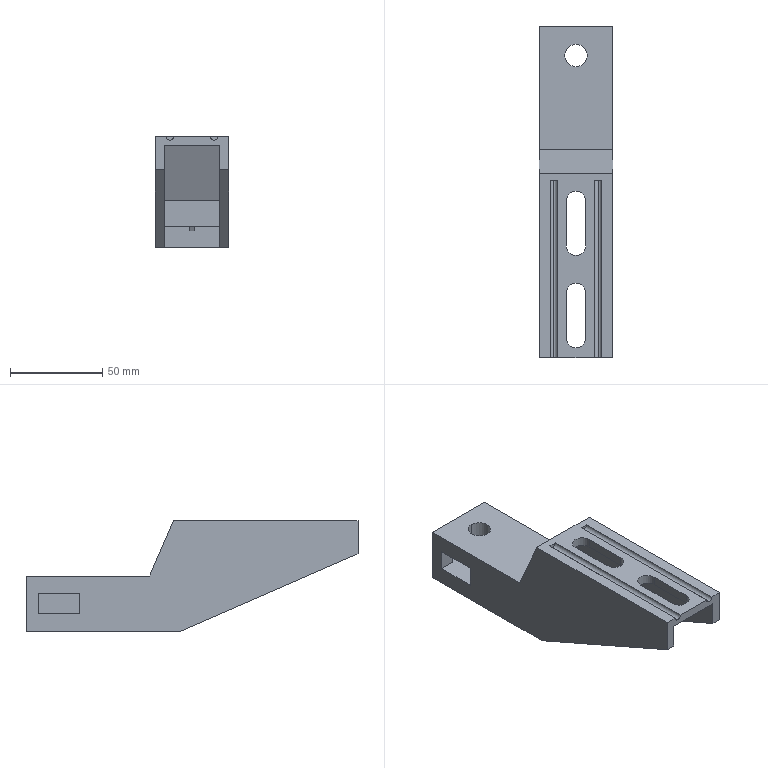Part | SolidWorks | features BaseBody 1 | 1 solid | 48 faces | box 40 x 180 x 60 mm | volume 106020 mm3 | plane 36 | cylinder 12 | commonest cylinder face diameters 4 x4 10.5 x4 12.2 x4
STEP:
#1=CARTESIAN_POINT('',(12.,96.,-2.));
#2=VERTEX_POINT('',#1);
#3=CARTESIAN_POINT('',(14.,96.,0.));
#4=VERTEX_POINT('',#3);
#5=CARTESIAN_POINT('',(12.,96.,0.));
#6=DIRECTION('',(0.,-1.,0.));
#7=DIRECTION('',(0.,0.,-1.));
#8=AXIS2_PLACEMENT_3D('',#5,#6,#7);
#9=CIRCLE('',#8,2.);
#10=EDGE_CURVE('',#2,#4,#9,.T.);
#11=ORIENTED_EDGE('',*,*,#10,.F.);
#12=CARTESIAN_POINT('',(12.,0.,-2.));
#13=VERTEX_POINT('',#12);
#14=CARTESIAN_POINT('',(12.,96.,-2.));
#15=DIRECTION('',(0.,-1.,0.));
#16=VECTOR('',#15,1000.);
#17=LINE('',#14,#16);
#18=EDGE_CURVE('',#2,#13,#17,.T.);
#19=ORIENTED_EDGE('',*,*,#18,.T.);
#20=CARTESIAN_POINT('',(14.,0.,0.));
#21=VERTEX_POINT('',#20);
#22=CARTESIAN_POINT('',(12.,0.,0.));
#23=DIRECTION('',(0.,-1.,0.));
#24=DIRECTION('',(0.,0.,-1.));
#25=AXIS2_PLACEMENT_3D('',#22,#23,#24);
#26=CIRCLE('',#25,2.);
#27=EDGE_CURVE('',#13,#21,#26,.T.);
#28=ORIENTED_EDGE('',*,*,#27,.T.);
#29=CARTESIAN_POINT('',(14.,0.,0.));
#30=DIRECTION('',(0.,1.,0.));
#31=VECTOR('',#30,1000.);
#32=LINE('',#29,#31);
#33=EDGE_CURVE('',#21,#4,#32,.T.);
#34=ORIENTED_EDGE('',*,*,#33,.T.);
#35=EDGE_LOOP('',(#11,#19,#28,#34));
#36=FACE_OUTER_BOUND('',#35,.T.);
#37=CARTESIAN_POINT('',(12.,96.,0.));
#38=DIRECTION('',(0.,-1.,0.));
#39=DIRECTION('',(0.,0.,-1.));
#40=AXIS2_PLACEMENT_3D('',#37,#38,#39);
#41=CYLINDRICAL_SURFACE('',#40,2.);
#42=ADVANCED_FACE('',(#36),#41,.F.);
#43=CARTESIAN_POINT('',(-12.,96.,-2.));
#44=VERTEX_POINT('',#43);
#45=CARTESIAN_POINT('',(-10.,96.,0.));
#46=VERTEX_POINT('',#45);
#47=CARTESIAN_POINT('',(-12.,96.,0.));
#48=DIRECTION('',(0.,-1.,0.));
#49=DIRECTION('',(0.,0.,-1.));
#50=AXIS2_PLACEMENT_3D('',#47,#48,#49);
#51=CIRCLE('',#50,2.);
#52=EDGE_CURVE('',#44,#46,#51,.T.);
#53=ORIENTED_EDGE('',*,*,#52,.F.);
#54=CARTESIAN_POINT('',(-12.,0.,-2.));
#55=VERTEX_POINT('',#54);
#56=CARTESIAN_POINT('',(-12.,96.,-2.));
#57=DIRECTION('',(0.,-1.,0.));
#58=VECTOR('',#57,1000.);
#59=LINE('',#56,#58);
#60=EDGE_CURVE('',#44,#55,#59,.T.);
#61=ORIENTED_EDGE('',*,*,#60,.T.);
#62=CARTESIAN_POINT('',(-10.,0.,0.));
#63=VERTEX_POINT('',#62);
#64=CARTESIAN_POINT('',(-12.,0.,0.));
#65=DIRECTION('',(0.,-1.,0.));
#66=DIRECTION('',(0.,0.,-1.));
#67=AXIS2_PLACEMENT_3D('',#64,#65,#66);
#68=CIRCLE('',#67,2.);
#69=EDGE_CURVE('',#55,#63,#68,.T.);
#70=ORIENTED_EDGE('',*,*,#69,.T.);
#71=CARTESIAN_POINT('',(-10.,0.,0.));
#72=DIRECTION('',(0.,1.,0.));
#73=VECTOR('',#72,1000.);
#74=LINE('',#71,#73);
#75=EDGE_CURVE('',#63,#46,#74,.T.);
#76=ORIENTED_EDGE('',*,*,#75,.T.);
#77=EDGE_LOOP('',(#53,#61,#70,#76));
#78=FACE_OUTER_BOUND('',#77,.T.);
#79=CARTESIAN_POINT('',(-12.,96.,0.));
#80=DIRECTION('',(0.,-1.,0.));
#81=DIRECTION('',(0.,0.,-1.));
#82=AXIS2_PLACEMENT_3D('',#79,#80,#81);
#83=CYLINDRICAL_SURFACE('',#82,2.);
#84=ADVANCED_FACE('',(#78),#83,.F.);
#85=CARTESIAN_POINT('',(0.,157.9,-50.6));
#86=VERTEX_POINT('',#85);
#87=CARTESIAN_POINT('',(0.,170.1,-50.6));
#88=VERTEX_POINT('',#87);
#89=CARTESIAN_POINT('',(0.,164.,-50.6));
#90=DIRECTION('',(0.,0.,-1.));
#91=DIRECTION('',(0.,1.,0.));
#92=AXIS2_PLACEMENT_3D('',#89,#90,#91);
#93=CIRCLE('',#92,6.1);
#94=EDGE_CURVE('',#86,#88,#93,.T.);
#95=ORIENTED_EDGE('',*,*,#94,.F.);
#96=CARTESIAN_POINT('',(0.,157.9,-60.));
#97=VERTEX_POINT('',#96);
#98=CARTESIAN_POINT('',(0.,157.9,0.));
#99=DIRECTION('',(0.,0.,-1.));
#100=VECTOR('',#99,1000.);
#101=LINE('',#98,#100);
#102=EDGE_CURVE('',#86,#97,#101,.T.);
#103=ORIENTED_EDGE('',*,*,#102,.T.);
#104=CARTESIAN_POINT('',(0.,170.1,-60.));
#105=VERTEX_POINT('',#104);
#106=CARTESIAN_POINT('',(0.,164.,-60.));
#107=DIRECTION('',(0.,0.,-1.));
#108=DIRECTION('',(0.,1.,0.));
#109=AXIS2_PLACEMENT_3D('',#106,#107,#108);
#110=CIRCLE('',#109,6.1);
#111=EDGE_CURVE('',#97,#105,#110,.T.);
#112=ORIENTED_EDGE('',*,*,#111,.T.);
#113=CARTESIAN_POINT('',(0.,170.1,0.));
#114=DIRECTION('',(0.,0.,-1.));
#115=VECTOR('',#114,1000.);
#116=LINE('',#113,#115);
#117=EDGE_CURVE('',#88,#105,#116,.T.);
#118=ORIENTED_EDGE('',*,*,#117,.F.);
#119=EDGE_LOOP('',(#95,#103,#112,#118));
#120=FACE_OUTER_BOUND('',#119,.T.);
#121=CARTESIAN_POINT('',(0.,164.,0.));
#122=DIRECTION('',(0.,0.,-1.));
#123=DIRECTION('',(0.,1.,0.));
#124=AXIS2_PLACEMENT_3D('',#121,#122,#123);
#125=CYLINDRICAL_SURFACE('',#124,6.1);
#126=ADVANCED_FACE('',(#120),#125,.F.);
#127=CARTESIAN_POINT('',(0.,170.1,-30.));
#128=VERTEX_POINT('',#127);
#129=CARTESIAN_POINT('',(0.,157.9,-30.));
#130=VERTEX_POINT('',#129);
#131=CARTESIAN_POINT('',(0.,164.,-30.));
#132=DIRECTION('',(0.,0.,1.));
#133=DIRECTION('',(0.,1.,0.));
#134=AXIS2_PLACEMENT_3D('',#131,#132,#133);
#135=CIRCLE('',#134,6.1);
#136=EDGE_CURVE('',#128,#130,#135,.T.);
#137=ORIENTED_EDGE('',*,*,#136,.T.);
#138=CARTESIAN_POINT('',(0.,157.9,-39.4));
#139=VERTEX_POINT('',#138);
#140=CARTESIAN_POINT('',(0.,157.9,0.));
#141=DIRECTION('',(0.,0.,-1.));
#142=VECTOR('',#141,1000.);
#143=LINE('',#140,#142);
#144=EDGE_CURVE('',#130,#139,#143,.T.);
#145=ORIENTED_EDGE('',*,*,#144,.T.);
#146=CARTESIAN_POINT('',(0.,170.1,-39.4));
#147=VERTEX_POINT('',#146);
#148=CARTESIAN_POINT('',(0.,164.,-39.4));
#149=DIRECTION('',(0.,0.,-1.));
#150=DIRECTION('',(0.,1.,0.));
#151=AXIS2_PLACEMENT_3D('',#148,#149,#150);
#152=CIRCLE('',#151,6.1);
#153=EDGE_CURVE('',#139,#147,#152,.T.);
#154=ORIENTED_EDGE('',*,*,#153,.T.);
#155=CARTESIAN_POINT('',(0.,170.1,0.));
#156=DIRECTION('',(0.,0.,-1.));
#157=VECTOR('',#156,1000.);
#158=LINE('',#155,#157);
#159=EDGE_CURVE('',#128,#147,#158,.T.);
#160=ORIENTED_EDGE('',*,*,#159,.F.);
#161=EDGE_LOOP('',(#137,#145,#154,#160));
#162=FACE_OUTER_BOUND('',#161,.T.);
#163=CARTESIAN_POINT('',(0.,164.,0.));
#164=DIRECTION('',(0.,0.,-1.));
#165=DIRECTION('',(0.,1.,0.));
#166=AXIS2_PLACEMENT_3D('',#163,#164,#165);
#167=CYLINDRICAL_SURFACE('',#166,6.1);
#168=ADVANCED_FACE('',(#162),#167,.F.);
#169=CARTESIAN_POINT('',(20.,96.,-60.));
#170=VERTEX_POINT('',#169);
#171=CARTESIAN_POINT('',(20.,0.,-18.));
#172=VERTEX_POINT('',#171);
#173=CARTESIAN_POINT('',(20.,96.,-60.));
#174=DIRECTION('',(0.,-0.9162,0.4008));
#175=VECTOR('',#174,1000.);
#176=LINE('',#173,#175);
#177=EDGE_CURVE('',#170,#172,#176,.T.);
#178=ORIENTED_EDGE('',*,*,#177,.F.);
#179=CARTESIAN_POINT('',(20.,180.,-60.));
#180=VERTEX_POINT('',#179);
#181=CARTESIAN_POINT('',(20.,0.,-60.));
#182=DIRECTION('',(0.,-1.,0.));
#183=VECTOR('',#182,1000.);
#184=LINE('',#181,#183);
#185=EDGE_CURVE('',#180,#170,#184,.T.);
#186=ORIENTED_EDGE('',*,*,#185,.F.);
#187=CARTESIAN_POINT('',(20.,180.,-30.));
#188=VERTEX_POINT('',#187);
#189=CARTESIAN_POINT('',(20.,180.,0.));
#190=DIRECTION('',(0.,0.,-1.));
#191=VECTOR('',#190,1000.);
#192=LINE('',#189,#191);
#193=EDGE_CURVE('',#188,#180,#192,.T.);
#194=ORIENTED_EDGE('',*,*,#193,.F.);
#195=CARTESIAN_POINT('',(20.,113.,-30.));
#196=VERTEX_POINT('',#195);
#197=CARTESIAN_POINT('',(20.,0.,-30.));
#198=DIRECTION('',(0.,1.,0.));
#199=VECTOR('',#198,1000.);
#200=LINE('',#197,#199);
#201=EDGE_CURVE('',#196,#188,#200,.T.);
#202=ORIENTED_EDGE('',*,*,#201,.F.);
#203=CARTESIAN_POINT('',(20.,100.,0.));
#204=VERTEX_POINT('',#203);
#205=CARTESIAN_POINT('',(20.,100.,0.));
#206=DIRECTION('',(0.,0.3976,-0.9176));
#207=VECTOR('',#206,1000.);
#208=LINE('',#205,#207);
#209=EDGE_CURVE('',#204,#196,#208,.T.);
#210=ORIENTED_EDGE('',*,*,#209,.F.);
#211=CARTESIAN_POINT('',(20.,0.,0.));
#212=VERTEX_POINT('',#211);
#213=CARTESIAN_POINT('',(20.,0.,0.));
#214=DIRECTION('',(0.,1.,0.));
#215=VECTOR('',#214,1000.);
#216=LINE('',#213,#215);
#217=EDGE_CURVE('',#212,#204,#216,.T.);
#218=ORIENTED_EDGE('',*,*,#217,.F.);
#219=CARTESIAN_POINT('',(20.,0.,0.));
#220=DIRECTION('',(0.,0.,1.));
#221=VECTOR('',#220,1000.);
#222=LINE('',#219,#221);
#223=EDGE_CURVE('',#172,#212,#222,.T.);
#224=ORIENTED_EDGE('',*,*,#223,.F.);
#225=EDGE_LOOP('',(#178,#186,#194,#202,#210,#218,#224));
#226=FACE_OUTER_BOUND('',#225,.T.);
#227=CARTESIAN_POINT('',(20.,0.,0.));
#228=DIRECTION('',(-1.,0.,0.));
#229=DIRECTION('',(0.,0.,1.));
#230=AXIS2_PLACEMENT_3D('',#227,#228,#229);
#231=PLANE('',#230);
#232=ADVANCED_FACE('',(#226),#231,.F.);
#233=CARTESIAN_POINT('',(10.,0.,0.));
#234=VERTEX_POINT('',#233);
#235=CARTESIAN_POINT('',(12.,0.,0.));
#236=DIRECTION('',(0.,-1.,0.));
#237=DIRECTION('',(0.,0.,-1.));
#238=AXIS2_PLACEMENT_3D('',#235,#236,#237);
#239=CIRCLE('',#238,2.);
#240=EDGE_CURVE('',#234,#13,#239,.T.);
#241=ORIENTED_EDGE('',*,*,#240,.F.);
#242=CARTESIAN_POINT('',(20.,0.,0.));
#243=DIRECTION('',(1.,0.,0.));
#244=VECTOR('',#243,1000.);
#245=LINE('',#242,#244);
#246=EDGE_CURVE('',#63,#234,#245,.T.);
#247=ORIENTED_EDGE('',*,*,#246,.F.);
#248=ORIENTED_EDGE('',*,*,#69,.F.);
#249=CARTESIAN_POINT('',(-14.,0.,0.));
#250=VERTEX_POINT('',#249);
#251=CARTESIAN_POINT('',(-12.,0.,0.));
#252=DIRECTION('',(0.,-1.,0.));
#253=DIRECTION('',(0.,0.,-1.));
#254=AXIS2_PLACEMENT_3D('',#251,#252,#253);
#255=CIRCLE('',#254,2.);
#256=EDGE_CURVE('',#250,#55,#255,.T.);
#257=ORIENTED_EDGE('',*,*,#256,.F.);
#258=CARTESIAN_POINT('',(-20.,0.,0.));
#259=VERTEX_POINT('',#258);
#260=CARTESIAN_POINT('',(20.,0.,0.));
#261=DIRECTION('',(1.,0.,0.));
#262=VECTOR('',#261,1000.);
#263=LINE('',#260,#262);
#264=EDGE_CURVE('',#259,#250,#263,.T.);
#265=ORIENTED_EDGE('',*,*,#264,.F.);
#266=CARTESIAN_POINT('',(-20.,0.,-18.));
#267=VERTEX_POINT('',#266);
#268=CARTESIAN_POINT('',(-20.,0.,-18.));
#269=DIRECTION('',(0.,0.,1.));
#270=VECTOR('',#269,1000.);
#271=LINE('',#268,#270);
#272=EDGE_CURVE('',#267,#259,#271,.T.);
#273=ORIENTED_EDGE('',*,*,#272,.F.);
#274=CARTESIAN_POINT('',(-15.,0.,-18.));
#275=VERTEX_POINT('',#274);
#276=CARTESIAN_POINT('',(20.,0.,-18.));
#277=DIRECTION('',(-1.,0.,0.));
#278=VECTOR('',#277,1000.);
#279=LINE('',#276,#278);
#280=EDGE_CURVE('',#275,#267,#279,.T.);
#281=ORIENTED_EDGE('',*,*,#280,.F.);
#282=CARTESIAN_POINT('',(-15.,0.,-5.));
#283=VERTEX_POINT('',#282);
#284=CARTESIAN_POINT('',(-15.,0.,-18.));
#285=DIRECTION('',(0.,0.,-1.));
#286=VECTOR('',#285,1000.);
#287=LINE('',#284,#286);
#288=EDGE_CURVE('',#283,#275,#287,.T.);
#289=ORIENTED_EDGE('',*,*,#288,.F.);
#290=CARTESIAN_POINT('',(15.,0.,-5.));
#291=VERTEX_POINT('',#290);
#292=CARTESIAN_POINT('',(20.,0.,-5.));
#293=DIRECTION('',(-1.,0.,0.));
#294=VECTOR('',#293,1000.);
#295=LINE('',#292,#294);
#296=EDGE_CURVE('',#291,#283,#295,.T.);
#297=ORIENTED_EDGE('',*,*,#296,.F.);
#298=CARTESIAN_POINT('',(15.,0.,-18.));
#299=VERTEX_POINT('',#298);
#300=CARTESIAN_POINT('',(15.,0.,-18.));
#301=DIRECTION('',(0.,0.,1.));
#302=VECTOR('',#301,1000.);
#303=LINE('',#300,#302);
#304=EDGE_CURVE('',#299,#291,#303,.T.);
#305=ORIENTED_EDGE('',*,*,#304,.F.);
#306=CARTESIAN_POINT('',(20.,0.,-18.));
#307=DIRECTION('',(-1.,0.,0.));
#308=VECTOR('',#307,1000.);
#309=LINE('',#306,#308);
#310=EDGE_CURVE('',#172,#299,#309,.T.);
#311=ORIENTED_EDGE('',*,*,#310,.F.);
#312=ORIENTED_EDGE('',*,*,#223,.T.);
#313=CARTESIAN_POINT('',(20.,0.,0.));
#314=DIRECTION('',(1.,0.,0.));
#315=VECTOR('',#314,1000.);
#316=LINE('',#313,#315);
#317=EDGE_CURVE('',#21,#212,#316,.T.);
#318=ORIENTED_EDGE('',*,*,#317,.F.);
#319=ORIENTED_EDGE('',*,*,#27,.F.);
#320=EDGE_LOOP('',(#241,#247,#248,#257,#265,#273,#281,#289,#297,#305,#311,#312,#318,#319));
#321=FACE_OUTER_BOUND('',#320,.T.);
#322=CARTESIAN_POINT('',(20.,0.,-18.));
#323=DIRECTION('',(0.,1.,0.));
#324=DIRECTION('',(0.,0.,1.));
#325=AXIS2_PLACEMENT_3D('',#322,#323,#324);
#326=PLANE('',#325);
#327=ADVANCED_FACE('',(#321),#326,.F.);
#328=CARTESIAN_POINT('',(15.,96.,-60.));
#329=VERTEX_POINT('',#328);
#330=CARTESIAN_POINT('',(15.,96.,-60.));
#331=DIRECTION('',(0.,-0.9162,0.4008));
#332=VECTOR('',#331,1000.);
#333=LINE('',#330,#332);
#334=EDGE_CURVE('',#329,#299,#333,.T.);
#335=ORIENTED_EDGE('',*,*,#334,.F.);
#336=CARTESIAN_POINT('',(20.,96.,-60.));
#337=DIRECTION('',(-1.,0.,0.));
#338=VECTOR('',#337,1000.);
#339=LINE('',#336,#338);
#340=EDGE_CURVE('',#170,#329,#339,.T.);
#341=ORIENTED_EDGE('',*,*,#340,.F.);
#342=ORIENTED_EDGE('',*,*,#177,.T.);
#343=ORIENTED_EDGE('',*,*,#310,.T.);
#344=EDGE_LOOP('',(#335,#341,#342,#343));
#345=FACE_OUTER_BOUND('',#344,.T.);
#346=CARTESIAN_POINT('',(20.,96.,-60.));
#347=DIRECTION('',(0.,0.4008,0.9162));
#348=DIRECTION('',(0.,-0.9162,0.4008));
#349=AXIS2_PLACEMENT_3D('',#346,#347,#348);
#350=PLANE('',#349);
#351=ADVANCED_FACE('',(#345),#350,.F.);
#352=CARTESIAN_POINT('',(0.,164.,-60.));
#353=DIRECTION('',(0.,0.,-1.));
#354=DIRECTION('',(0.,1.,0.));
#355=AXIS2_PLACEMENT_3D('',#352,#353,#354);
#356=CIRCLE('',#355,6.1);
#357=EDGE_CURVE('',#105,#97,#356,.T.);
#358=ORIENTED_EDGE('',*,*,#357,.F.);
#359=ORIENTED_EDGE('',*,*,#111,.F.);
#360=EDGE_LOOP('',(#358,#359));
#361=FACE_BOUND('',#360,.T.);
#362=CARTESIAN_POINT('',(-20.,96.,-60.));
#363=VERTEX_POINT('',#362);
#364=CARTESIAN_POINT('',(-15.,96.,-60.));
#365=VERTEX_POINT('',#364);
#366=CARTESIAN_POINT('',(20.,96.,-60.));
#367=DIRECTION('',(1.,0.,0.));
#368=VECTOR('',#367,1000.);
#369=LINE('',#366,#368);
#370=EDGE_CURVE('',#363,#365,#369,.T.);
#371=ORIENTED_EDGE('',*,*,#370,.F.);
#372=CARTESIAN_POINT('',(-20.,180.,-60.));
#373=VERTEX_POINT('',#372);
#374=CARTESIAN_POINT('',(-20.,180.,-60.));
#375=DIRECTION('',(0.,-1.,0.));
#376=VECTOR('',#375,1000.);
#377=LINE('',#374,#376);
#378=EDGE_CURVE('',#373,#363,#377,.T.);
#379=ORIENTED_EDGE('',*,*,#378,.F.);
#380=CARTESIAN_POINT('',(20.,180.,-60.));
#381=DIRECTION('',(-1.,0.,0.));
#382=VECTOR('',#381,1000.);
#383=LINE('',#380,#382);
#384=EDGE_CURVE('',#180,#373,#383,.T.);
#385=ORIENTED_EDGE('',*,*,#384,.F.);
#386=ORIENTED_EDGE('',*,*,#185,.T.);
#387=ORIENTED_EDGE('',*,*,#340,.T.);
#388=CARTESIAN_POINT('',(15.,147.,-60.));
#389=VERTEX_POINT('',#388);
#390=CARTESIAN_POINT('',(15.,180.,-60.));
#391=DIRECTION('',(0.,-1.,0.));
#392=VECTOR('',#391,1000.);
#393=LINE('',#390,#392);
#394=EDGE_CURVE('',#389,#329,#393,.T.);
#395=ORIENTED_EDGE('',*,*,#394,.F.);
#396=CARTESIAN_POINT('',(-15.,147.,-60.));
#397=VERTEX_POINT('',#396);
#398=CARTESIAN_POINT('',(20.,147.,-60.));
#399=DIRECTION('',(1.,0.,0.));
#400=VECTOR('',#399,1000.);
#401=LINE('',#398,#400);
#402=EDGE_CURVE('',#397,#389,#401,.T.);
#403=ORIENTED_EDGE('',*,*,#402,.F.);
#404=CARTESIAN_POINT('',(-15.,180.,-60.));
#405=DIRECTION('',(0.,1.,0.));
#406=VECTOR('',#405,1000.);
#407=LINE('',#404,#406);
#408=EDGE_CURVE('',#365,#397,#407,.T.);
#409=ORIENTED_EDGE('',*,*,#408,.F.);
#410=EDGE_LOOP('',(#371,#379,#385,#386,#387,#395,#403,#409));
#411=FACE_OUTER_BOUND('',#410,.T.);
#412=CARTESIAN_POINT('',(20.,180.,-60.));
#413=DIRECTION('',(0.,0.,1.));
#414=DIRECTION('',(0.,-1.,0.));
#415=AXIS2_PLACEMENT_3D('',#412,#413,#414);
#416=PLANE('',#415);
#417=ADVANCED_FACE('',(#361,#411),#416,.F.);
#418=CARTESIAN_POINT('',(-11.5,180.,-50.6));
#419=VERTEX_POINT('',#418);
#420=CARTESIAN_POINT('',(-11.5,180.,-39.4));
#421=VERTEX_POINT('',#420);
#422=CARTESIAN_POINT('',(-11.5,180.,-30.));
#423=DIRECTION('',(0.,0.,1.));
#424=VECTOR('',#423,1000.);
#425=LINE('',#422,#424);
#426=EDGE_CURVE('',#419,#421,#425,.T.);
#427=ORIENTED_EDGE('',*,*,#426,.F.);
#428=CARTESIAN_POINT('',(11.5,180.,-50.6));
#429=VERTEX_POINT('',#428);
#430=CARTESIAN_POINT('',(20.,180.,-50.6));
#431=DIRECTION('',(-1.,0.,0.));
#432=VECTOR('',#431,1000.);
#433=LINE('',#430,#432);
#434=EDGE_CURVE('',#429,#419,#433,.T.);
#435=ORIENTED_EDGE('',*,*,#434,.F.);
#436=CARTESIAN_POINT('',(11.5,180.,-39.4));
#437=VERTEX_POINT('',#436);
#438=CARTESIAN_POINT('',(11.5,180.,-30.));
#439=DIRECTION('',(0.,0.,-1.));
#440=VECTOR('',#439,1000.);
#441=LINE('',#438,#440);
#442=EDGE_CURVE('',#437,#429,#441,.T.);
#443=ORIENTED_EDGE('',*,*,#442,.F.);
#444=CARTESIAN_POINT('',(20.,180.,-39.4));
#445=DIRECTION('',(1.,0.,0.));
#446=VECTOR('',#445,1000.);
#447=LINE('',#444,#446);
#448=EDGE_CURVE('',#421,#437,#447,.T.);
#449=ORIENTED_EDGE('',*,*,#448,.F.);
#450=EDGE_LOOP('',(#427,#435,#443,#449));
#451=FACE_BOUND('',#450,.T.);
#452=CARTESIAN_POINT('',(-20.,180.,-30.));
#453=VERTEX_POINT('',#452);
#454=CARTESIAN_POINT('',(20.,180.,-30.));
#455=DIRECTION('',(-1.,0.,0.));
#456=VECTOR('',#455,1000.);
#457=LINE('',#454,#456);
#458=EDGE_CURVE('',#188,#453,#457,.T.);
#459=ORIENTED_EDGE('',*,*,#458,.F.);
#460=ORIENTED_EDGE('',*,*,#193,.T.);
#461=ORIENTED_EDGE('',*,*,#384,.T.);
#462=CARTESIAN_POINT('',(-20.,180.,-30.));
#463=DIRECTION('',(0.,0.,-1.));
#464=VECTOR('',#463,1000.);
#465=LINE('',#462,#464);
#466=EDGE_CURVE('',#453,#373,#465,.T.);
#467=ORIENTED_EDGE('',*,*,#466,.F.);
#468=EDGE_LOOP('',(#459,#460,#461,#467));
#469=FACE_OUTER_BOUND('',#468,.T.);
#470=CARTESIAN_POINT('',(20.,180.,-30.));
#471=DIRECTION('',(0.,-1.,0.));
#472=DIRECTION('',(0.,0.,-1.));
#473=AXIS2_PLACEMENT_3D('',#470,#471,#472);
#474=PLANE('',#473);
#475=ADVANCED_FACE('',(#451,#469),#474,.F.);
#476=ORIENTED_EDGE('',*,*,#136,.F.);
#477=CARTESIAN_POINT('',(0.,164.,-30.));
#478=DIRECTION('',(0.,0.,1.));
#479=DIRECTION('',(0.,1.,0.));
#480=AXIS2_PLACEMENT_3D('',#477,#478,#479);
#481=CIRCLE('',#480,6.1);
#482=EDGE_CURVE('',#130,#128,#481,.T.);
#483=ORIENTED_EDGE('',*,*,#482,.F.);
#484=EDGE_LOOP('',(#476,#483));
#485=FACE_BOUND('',#484,.T.);
#486=CARTESIAN_POINT('',(-20.,113.,-30.));
#487=VERTEX_POINT('',#486);
#488=CARTESIAN_POINT('',(20.,113.,-30.));
#489=DIRECTION('',(-1.,0.,0.));
#490=VECTOR('',#489,1000.);
#491=LINE('',#488,#490);
#492=EDGE_CURVE('',#196,#487,#491,.T.);
#493=ORIENTED_EDGE('',*,*,#492,.F.);
#494=ORIENTED_EDGE('',*,*,#201,.T.);
#495=ORIENTED_EDGE('',*,*,#458,.T.);
#496=CARTESIAN_POINT('',(-20.,113.,-30.));
#497=DIRECTION('',(0.,1.,0.));
#498=VECTOR('',#497,1000.);
#499=LINE('',#496,#498);
#500=EDGE_CURVE('',#487,#453,#499,.T.);
#501=ORIENTED_EDGE('',*,*,#500,.F.);
#502=EDGE_LOOP('',(#493,#494,#495,#501));
#503=FACE_OUTER_BOUND('',#502,.T.);
#504=CARTESIAN_POINT('',(20.,113.,-30.));
#505=DIRECTION('',(0.,0.,-1.));
#506=DIRECTION('',(-1.,0.,0.));
#507=AXIS2_PLACEMENT_3D('',#504,#505,#506);
#508=PLANE('',#507);
#509=ADVANCED_FACE('',(#485,#503),#508,.F.);
#510=CARTESIAN_POINT('',(-20.,100.,0.));
#511=VERTEX_POINT('',#510);
#512=CARTESIAN_POINT('',(20.,100.,0.));
#513=DIRECTION('',(-1.,0.,0.));
#514=VECTOR('',#513,1000.);
#515=LINE('',#512,#514);
#516=EDGE_CURVE('',#204,#511,#515,.T.);
#517=ORIENTED_EDGE('',*,*,#516,.F.);
#518=ORIENTED_EDGE('',*,*,#209,.T.);
#519=ORIENTED_EDGE('',*,*,#492,.T.);
#520=CARTESIAN_POINT('',(-20.,100.,0.));
#521=DIRECTION('',(0.,0.3976,-0.9176));
#522=VECTOR('',#521,1000.);
#523=LINE('',#520,#522);
#524=EDGE_CURVE('',#511,#487,#523,.T.);
#525=ORIENTED_EDGE('',*,*,#524,.F.);
#526=EDGE_LOOP('',(#517,#518,#519,#525));
#527=FACE_OUTER_BOUND('',#526,.T.);
#528=CARTESIAN_POINT('',(20.,100.,0.));
#529=DIRECTION('',(0.,-0.9176,-0.3976));
#530=DIRECTION('',(0.,0.3976,-0.9176));
#531=AXIS2_PLACEMENT_3D('',#528,#529,#530);
#532=PLANE('',#531);
#533=ADVANCED_FACE('',(#527),#532,.F.);
#534=CARTESIAN_POINT('',(-5.25,10.75,0.));
#535=VERTEX_POINT('',#534);
#536=CARTESIAN_POINT('',(5.25,10.75,0.));
#537=VERTEX_POINT('',#536);
#538=CARTESIAN_POINT('',(0.,10.75,0.));
#539=DIRECTION('',(0.,0.,1.));
#540=DIRECTION('',(1.,0.,0.));
#541=AXIS2_PLACEMENT_3D('',#538,#539,#540);
#542=CIRCLE('',#541,5.25);
#543=EDGE_CURVE('',#535,#537,#542,.T.);
#544=ORIENTED_EDGE('',*,*,#543,.F.);
#545=CARTESIAN_POINT('',(-5.25,35.25,0.));
#546=VERTEX_POINT('',#545);
#547=CARTESIAN_POINT('',(-5.25,0.,0.));
#548=DIRECTION('',(0.,-1.,0.));
#549=VECTOR('',#548,1000.);
#550=LINE('',#547,#549);
#551=EDGE_CURVE('',#546,#535,#550,.T.);
#552=ORIENTED_EDGE('',*,*,#551,.F.);
#553=CARTESIAN_POINT('',(5.25,35.25,0.));
#554=VERTEX_POINT('',#553);
#555=CARTESIAN_POINT('',(0.,35.25,0.));
#556=DIRECTION('',(0.,0.,1.));
#557=DIRECTION('',(1.,0.,0.));
#558=AXIS2_PLACEMENT_3D('',#555,#556,#557);
#559=CIRCLE('',#558,5.25);
#560=EDGE_CURVE('',#554,#546,#559,.T.);
#561=ORIENTED_EDGE('',*,*,#560,.F.);
#562=CARTESIAN_POINT('',(5.25,0.,0.));
#563=DIRECTION('',(0.,1.,0.));
#564=VECTOR('',#563,1000.);
#565=LINE('',#562,#564);
#566=EDGE_CURVE('',#537,#554,#565,.T.);
#567=ORIENTED_EDGE('',*,*,#566,.F.);
#568=EDGE_LOOP('',(#544,#552,#561,#567));
#569=FACE_BOUND('',#568,.T.);
#570=CARTESIAN_POINT('',(-5.25,60.75,0.));
#571=VERTEX_POINT('',#570);
#572=CARTESIAN_POINT('',(5.25,60.75,0.));
#573=VERTEX_POINT('',#572);
#574=CARTESIAN_POINT('',(0.,60.75,0.));
#575=DIRECTION('',(0.,0.,1.));
#576=DIRECTION('',(1.,0.,0.));
#577=AXIS2_PLACEMENT_3D('',#574,#575,#576);
#578=CIRCLE('',#577,5.25);
#579=EDGE_CURVE('',#571,#573,#578,.T.);
#580=ORIENTED_EDGE('',*,*,#579,.F.);
#581=CARTESIAN_POINT('',(-5.25,85.25,0.));
#582=VERTEX_POINT('',#581);
#583=CARTESIAN_POINT('',(-5.25,0.,0.));
#584=DIRECTION('',(0.,-1.,0.));
#585=VECTOR('',#584,1000.);
#586=LINE('',#583,#585);
#587=EDGE_CURVE('',#582,#571,#586,.T.);
#588=ORIENTED_EDGE('',*,*,#587,.F.);
#589=CARTESIAN_POINT('',(5.25,85.25,0.));
#590=VERTEX_POINT('',#589);
#591=CARTESIAN_POINT('',(0.,85.25,0.));
#592=DIRECTION('',(0.,0.,1.));
#593=DIRECTION('',(1.,0.,0.));
#594=AXIS2_PLACEMENT_3D('',#591,#592,#593);
#595=CIRCLE('',#594,5.25);
#596=EDGE_CURVE('',#590,#582,#595,.T.);
#597=ORIENTED_EDGE('',*,*,#596,.F.);
#598=CARTESIAN_POINT('',(5.25,0.,0.));
#599=DIRECTION('',(0.,1.,0.));
#600=VECTOR('',#599,1000.);
#601=LINE('',#598,#600);
#602=EDGE_CURVE('',#573,#590,#601,.T.);
#603=ORIENTED_EDGE('',*,*,#602,.F.);
#604=EDGE_LOOP('',(#580,#588,#597,#603));
#605=FACE_BOUND('',#604,.T.);
#606=ORIENTED_EDGE('',*,*,#33,.F.);
#607=ORIENTED_EDGE('',*,*,#317,.T.);
#608=ORIENTED_EDGE('',*,*,#217,.T.);
#609=ORIENTED_EDGE('',*,*,#516,.T.);
#610=CARTESIAN_POINT('',(-20.,0.,0.));
#611=DIRECTION('',(0.,1.,0.));
#612=VECTOR('',#611,1000.);
#613=LINE('',#610,#612);
#614=EDGE_CURVE('',#259,#511,#613,.T.);
#615=ORIENTED_EDGE('',*,*,#614,.F.);
#616=ORIENTED_EDGE('',*,*,#264,.T.);
#617=CARTESIAN_POINT('',(-14.,96.,0.));
#618=VERTEX_POINT('',#617);
#619=CARTESIAN_POINT('',(-14.,0.,0.));
#620=DIRECTION('',(0.,-1.,0.));
#621=VECTOR('',#620,1000.);
#622=LINE('',#619,#621);
#623=EDGE_CURVE('',#618,#250,#622,.T.);
#624=ORIENTED_EDGE('',*,*,#623,.F.);
#625=CARTESIAN_POINT('',(20.,96.,0.));
#626=DIRECTION('',(-1.,0.,0.));
#627=VECTOR('',#626,1000.);
#628=LINE('',#625,#627);
#629=EDGE_CURVE('',#46,#618,#628,.T.);
#630=ORIENTED_EDGE('',*,*,#629,.F.);
#631=ORIENTED_EDGE('',*,*,#75,.F.);
#632=ORIENTED_EDGE('',*,*,#246,.T.);
#633=CARTESIAN_POINT('',(10.,96.,0.));
#634=VERTEX_POINT('',#633);
#635=CARTESIAN_POINT('',(10.,0.,0.));
#636=DIRECTION('',(0.,-1.,0.));
#637=VECTOR('',#636,1000.);
#638=LINE('',#635,#637);
#639=EDGE_CURVE('',#634,#234,#638,.T.);
#640=ORIENTED_EDGE('',*,*,#639,.F.);
#641=CARTESIAN_POINT('',(20.,96.,0.));
#642=DIRECTION('',(-1.,0.,0.));
#643=VECTOR('',#642,1000.);
#644=LINE('',#641,#643);
#645=EDGE_CURVE('',#4,#634,#644,.T.);
#646=ORIENTED_EDGE('',*,*,#645,.F.);
#647=EDGE_LOOP('',(#606,#607,#608,#609,#615,#616,#624,#630,#631,#632,#640,#646));
#648=FACE_OUTER_BOUND('',#647,.T.);
#649=CARTESIAN_POINT('',(20.,0.,0.));
#650=DIRECTION('',(0.,0.,-1.));
#651=DIRECTION('',(-1.,0.,0.));
#652=AXIS2_PLACEMENT_3D('',#649,#650,#651);
#653=PLANE('',#652);
#654=ADVANCED_FACE('',(#569,#605,#648),#653,.F.);
#655=ORIENTED_EDGE('',*,*,#18,.F.);
#656=CARTESIAN_POINT('',(12.,96.,0.));
#657=DIRECTION('',(0.,-1.,0.));
#658=DIRECTION('',(0.,0.,-1.));
#659=AXIS2_PLACEMENT_3D('',#656,#657,#658);
#660=CIRCLE('',#659,2.);
#661=EDGE_CURVE('',#634,#2,#660,.T.);
#662=ORIENTED_EDGE('',*,*,#661,.F.);
#663=ORIENTED_EDGE('',*,*,#639,.T.);
#664=ORIENTED_EDGE('',*,*,#240,.T.);
#665=EDGE_LOOP('',(#655,#662,#663,#664));
#666=FACE_OUTER_BOUND('',#665,.T.);
#667=CARTESIAN_POINT('',(12.,96.,0.));
#668=DIRECTION('',(0.,-1.,0.));
#669=DIRECTION('',(0.,0.,-1.));
#670=AXIS2_PLACEMENT_3D('',#667,#668,#669);
#671=CYLINDRICAL_SURFACE('',#670,2.);
#672=ADVANCED_FACE('',(#666),#671,.F.);
#673=ORIENTED_EDGE('',*,*,#60,.F.);
#674=CARTESIAN_POINT('',(-12.,96.,0.));
#675=DIRECTION('',(0.,-1.,0.));
#676=DIRECTION('',(0.,0.,-1.));
#677=AXIS2_PLACEMENT_3D('',#674,#675,#676);
#678=CIRCLE('',#677,2.);
#679=EDGE_CURVE('',#618,#44,#678,.T.);
#680=ORIENTED_EDGE('',*,*,#679,.F.);
#681=ORIENTED_EDGE('',*,*,#623,.T.);
#682=ORIENTED_EDGE('',*,*,#256,.T.);
#683=EDGE_LOOP('',(#673,#680,#681,#682));
#684=FACE_OUTER_BOUND('',#683,.T.);
#685=CARTESIAN_POINT('',(-12.,96.,0.));
#686=DIRECTION('',(0.,-1.,0.));
#687=DIRECTION('',(0.,0.,-1.));
#688=AXIS2_PLACEMENT_3D('',#685,#686,#687);
#689=CYLINDRICAL_SURFACE('',#688,2.);
#690=ADVANCED_FACE('',(#684),#689,.F.);
#691=CARTESIAN_POINT('',(-20.,173.,-39.4));
#692=VERTEX_POINT('',#691);
#693=CARTESIAN_POINT('',(-20.,151.,-39.4));
#694=VERTEX_POINT('',#693);
#695=CARTESIAN_POINT('',(-20.,0.,-39.4));
#696=DIRECTION('',(0.,-1.,0.));
#697=VECTOR('',#696,1000.);
#698=LINE('',#695,#697);
#699=EDGE_CURVE('',#692,#694,#698,.T.);
#700=ORIENTED_EDGE('',*,*,#699,.T.);
#701=CARTESIAN_POINT('',(-20.,151.,-50.6));
#702=VERTEX_POINT('',#701);
#703=CARTESIAN_POINT('',(-20.,151.,0.));
#704=DIRECTION('',(0.,0.,-1.));
#705=VECTOR('',#704,1000.);
#706=LINE('',#703,#705);
#707=EDGE_CURVE('',#694,#702,#706,.T.);
#708=ORIENTED_EDGE('',*,*,#707,.T.);
#709=CARTESIAN_POINT('',(-20.,173.,-50.6));
#710=VERTEX_POINT('',#709);
#711=CARTESIAN_POINT('',(-20.,0.,-50.6));
#712=DIRECTION('',(0.,1.,0.));
#713=VECTOR('',#712,1000.);
#714=LINE('',#711,#713);
#715=EDGE_CURVE('',#702,#710,#714,.T.);
#716=ORIENTED_EDGE('',*,*,#715,.T.);
#717=CARTESIAN_POINT('',(-20.,173.,0.));
#718=DIRECTION('',(0.,0.,1.));
#719=VECTOR('',#718,1000.);
#720=LINE('',#717,#719);
#721=EDGE_CURVE('',#710,#692,#720,.T.);
#722=ORIENTED_EDGE('',*,*,#721,.T.);
#723=EDGE_LOOP('',(#700,#708,#716,#722));
#724=FACE_BOUND('',#723,.T.);
#725=ORIENTED_EDGE('',*,*,#378,.T.);
#726=CARTESIAN_POINT('',(-20.,96.,-60.));
#727=DIRECTION('',(0.,-0.9162,0.4008));
#728=VECTOR('',#727,1000.);
#729=LINE('',#726,#728);
#730=EDGE_CURVE('',#363,#267,#729,.T.);
#731=ORIENTED_EDGE('',*,*,#730,.T.);
#732=ORIENTED_EDGE('',*,*,#272,.T.);
#733=ORIENTED_EDGE('',*,*,#614,.T.);
#734=ORIENTED_EDGE('',*,*,#524,.T.);
#735=ORIENTED_EDGE('',*,*,#500,.T.);
#736=ORIENTED_EDGE('',*,*,#466,.T.);
#737=EDGE_LOOP('',(#725,#731,#732,#733,#734,#735,#736));
#738=FACE_OUTER_BOUND('',#737,.T.);
#739=CARTESIAN_POINT('',(-20.,0.,0.));
#740=DIRECTION('',(-1.,0.,0.));
#741=DIRECTION('',(0.,0.,1.));
#742=AXIS2_PLACEMENT_3D('',#739,#740,#741);
#743=PLANE('',#742);
#744=ADVANCED_FACE('',(#724,#738),#743,.T.);
#745=ORIENTED_EDGE('',*,*,#280,.T.);
#746=ORIENTED_EDGE('',*,*,#730,.F.);
#747=ORIENTED_EDGE('',*,*,#370,.T.);
#748=CARTESIAN_POINT('',(-15.,96.,-60.));
#749=DIRECTION('',(0.,0.9162,-0.4008));
#750=VECTOR('',#749,1000.);
#751=LINE('',#748,#750);
#752=EDGE_CURVE('',#275,#365,#751,.T.);
#753=ORIENTED_EDGE('',*,*,#752,.F.);
#754=EDGE_LOOP('',(#745,#746,#747,#753));
#755=FACE_OUTER_BOUND('',#754,.T.);
#756=CARTESIAN_POINT('',(20.,96.,-60.));
#757=DIRECTION('',(0.,0.4008,0.9162));
#758=DIRECTION('',(0.,-0.9162,0.4008));
#759=AXIS2_PLACEMENT_3D('',#756,#757,#758);
#760=PLANE('',#759);
#761=ADVANCED_FACE('',(#755),#760,.F.);
#762=CARTESIAN_POINT('',(-15.,109.4,-48.633));
#763=VERTEX_POINT('',#762);
#764=CARTESIAN_POINT('',(-15.,111.6,-48.633));
#765=VERTEX_POINT('',#764);
#766=CARTESIAN_POINT('',(-15.,0.,-48.633));
#767=DIRECTION('',(0.,1.,0.));
#768=VECTOR('',#767,1000.);
#769=LINE('',#766,#768);
#770=EDGE_CURVE('',#763,#765,#769,.T.);
#771=ORIENTED_EDGE('',*,*,#770,.F.);
#772=CARTESIAN_POINT('',(-15.,109.4,-34.633));
#773=VERTEX_POINT('',#772);
#774=CARTESIAN_POINT('',(-15.,109.4,0.));
#775=DIRECTION('',(0.,0.,-1.));
#776=VECTOR('',#775,1000.);
#777=LINE('',#774,#776);
#778=EDGE_CURVE('',#773,#763,#777,.T.);
#779=ORIENTED_EDGE('',*,*,#778,.F.);
#780=CARTESIAN_POINT('',(-15.,109.558,-34.633));
#781=VERTEX_POINT('',#780);
#782=CARTESIAN_POINT('',(-15.,111.6,-34.633));
#783=DIRECTION('',(0.,-1.,0.));
#784=VECTOR('',#783,1000.);
#785=LINE('',#782,#784);
#786=EDGE_CURVE('',#781,#773,#785,.T.);
#787=ORIENTED_EDGE('',*,*,#786,.F.);
#788=CARTESIAN_POINT('',(-15.,96.717,-5.));
#789=VERTEX_POINT('',#788);
#790=CARTESIAN_POINT('',(-15.,96.717,-5.));
#791=DIRECTION('',(0.,0.3976,-0.9176));
#792=VECTOR('',#791,1000.);
#793=LINE('',#790,#792);
#794=EDGE_CURVE('',#789,#781,#793,.T.);
#795=ORIENTED_EDGE('',*,*,#794,.F.);
#796=CARTESIAN_POINT('',(-15.,0.,-5.));
#797=DIRECTION('',(0.,1.,0.));
#798=VECTOR('',#797,1000.);
#799=LINE('',#796,#798);
#800=EDGE_CURVE('',#283,#789,#799,.T.);
#801=ORIENTED_EDGE('',*,*,#800,.F.);
#802=ORIENTED_EDGE('',*,*,#288,.T.);
#803=ORIENTED_EDGE('',*,*,#752,.T.);
#804=ORIENTED_EDGE('',*,*,#408,.T.);
#805=CARTESIAN_POINT('',(-15.,147.,-35.));
#806=VERTEX_POINT('',#805);
#807=CARTESIAN_POINT('',(-15.,147.,0.));
#808=DIRECTION('',(0.,0.,-1.));
#809=VECTOR('',#808,1000.);
#810=LINE('',#807,#809);
#811=EDGE_CURVE('',#806,#397,#810,.T.);
#812=ORIENTED_EDGE('',*,*,#811,.F.);
#813=CARTESIAN_POINT('',(-15.,111.6,-35.));
#814=VERTEX_POINT('',#813);
#815=CARTESIAN_POINT('',(-15.,0.,-35.));
#816=DIRECTION('',(0.,1.,0.));
#817=VECTOR('',#816,1000.);
#818=LINE('',#815,#817);
#819=EDGE_CURVE('',#814,#806,#818,.T.);
#820=ORIENTED_EDGE('',*,*,#819,.F.);
#821=CARTESIAN_POINT('',(-15.,111.6,0.));
#822=DIRECTION('',(0.,0.,1.));
#823=VECTOR('',#822,1000.);
#824=LINE('',#821,#823);
#825=EDGE_CURVE('',#765,#814,#824,.T.);
#826=ORIENTED_EDGE('',*,*,#825,.F.);
#827=EDGE_LOOP('',(#771,#779,#787,#795,#801,#802,#803,#804,#812,#820,#826));
#828=FACE_OUTER_BOUND('',#827,.T.);
#829=CARTESIAN_POINT('',(-15.,0.,0.));
#830=DIRECTION('',(-1.,0.,0.));
#831=DIRECTION('',(0.,0.,1.));
#832=AXIS2_PLACEMENT_3D('',#829,#830,#831);
#833=PLANE('',#832);
#834=ADVANCED_FACE('',(#828),#833,.F.);
#835=CARTESIAN_POINT('',(5.25,35.25,-5.));
#836=VERTEX_POINT('',#835);
#837=CARTESIAN_POINT('',(-5.25,35.25,-5.));
#838=VERTEX_POINT('',#837);
#839=CARTESIAN_POINT('',(0.,35.25,-5.));
#840=DIRECTION('',(0.,0.,1.));
#841=DIRECTION('',(1.,0.,0.));
#842=AXIS2_PLACEMENT_3D('',#839,#840,#841);
#843=CIRCLE('',#842,5.25);
#844=EDGE_CURVE('',#836,#838,#843,.T.);
#845=ORIENTED_EDGE('',*,*,#844,.T.);
#846=CARTESIAN_POINT('',(-5.25,10.75,-5.));
#847=VERTEX_POINT('',#846);
#848=CARTESIAN_POINT('',(-5.25,0.,-5.));
#849=DIRECTION('',(0.,-1.,0.));
#850=VECTOR('',#849,1000.);
#851=LINE('',#848,#850);
#852=EDGE_CURVE('',#838,#847,#851,.T.);
#853=ORIENTED_EDGE('',*,*,#852,.T.);
#854=CARTESIAN_POINT('',(5.25,10.75,-5.));
#855=VERTEX_POINT('',#854);
#856=CARTESIAN_POINT('',(0.,10.75,-5.));
#857=DIRECTION('',(0.,0.,1.));
#858=DIRECTION('',(1.,0.,0.));
#859=AXIS2_PLACEMENT_3D('',#856,#857,#858);
#860=CIRCLE('',#859,5.25);
#861=EDGE_CURVE('',#847,#855,#860,.T.);
#862=ORIENTED_EDGE('',*,*,#861,.T.);
#863=CARTESIAN_POINT('',(5.25,0.,-5.));
#864=DIRECTION('',(0.,1.,0.));
#865=VECTOR('',#864,1000.);
#866=LINE('',#863,#865);
#867=EDGE_CURVE('',#855,#836,#866,.T.);
#868=ORIENTED_EDGE('',*,*,#867,.T.);
#869=EDGE_LOOP('',(#845,#853,#862,#868));
#870=FACE_BOUND('',#869,.T.);
#871=CARTESIAN_POINT('',(5.25,85.25,-5.));
#872=VERTEX_POINT('',#871);
#873=CARTESIAN_POINT('',(-5.25,85.25,-5.));
#874=VERTEX_POINT('',#873);
#875=CARTESIAN_POINT('',(0.,85.25,-5.));
#876=DIRECTION('',(0.,0.,1.));
#877=DIRECTION('',(1.,0.,0.));
#878=AXIS2_PLACEMENT_3D('',#875,#876,#877);
#879=CIRCLE('',#878,5.25);
#880=EDGE_CURVE('',#872,#874,#879,.T.);
#881=ORIENTED_EDGE('',*,*,#880,.T.);
#882=CARTESIAN_POINT('',(-5.25,60.75,-5.));
#883=VERTEX_POINT('',#882);
#884=CARTESIAN_POINT('',(-5.25,0.,-5.));
#885=DIRECTION('',(0.,-1.,0.));
#886=VECTOR('',#885,1000.);
#887=LINE('',#884,#886);
#888=EDGE_CURVE('',#874,#883,#887,.T.);
#889=ORIENTED_EDGE('',*,*,#888,.T.);
#890=CARTESIAN_POINT('',(5.25,60.75,-5.));
#891=VERTEX_POINT('',#890);
#892=CARTESIAN_POINT('',(0.,60.75,-5.));
#893=DIRECTION('',(0.,0.,1.));
#894=DIRECTION('',(1.,0.,0.));
#895=AXIS2_PLACEMENT_3D('',#892,#893,#894);
#896=CIRCLE('',#895,5.25);
#897=EDGE_CURVE('',#883,#891,#896,.T.);
#898=ORIENTED_EDGE('',*,*,#897,.T.);
#899=CARTESIAN_POINT('',(5.25,0.,-5.));
#900=DIRECTION('',(0.,1.,0.));
#901=VECTOR('',#900,1000.);
#902=LINE('',#899,#901);
#903=EDGE_CURVE('',#891,#872,#902,.T.);
#904=ORIENTED_EDGE('',*,*,#903,.T.);
#905=EDGE_LOOP('',(#881,#889,#898,#904));
#906=FACE_BOUND('',#905,.T.);
#907=CARTESIAN_POINT('',(15.,96.717,-5.));
#908=VERTEX_POINT('',#907);
#909=CARTESIAN_POINT('',(15.,0.,-5.));
#910=DIRECTION('',(0.,-1.,0.));
#911=VECTOR('',#910,1000.);
#912=LINE('',#909,#911);
#913=EDGE_CURVE('',#908,#291,#912,.T.);
#914=ORIENTED_EDGE('',*,*,#913,.T.);
#915=ORIENTED_EDGE('',*,*,#296,.T.);
#916=ORIENTED_EDGE('',*,*,#800,.T.);
#917=CARTESIAN_POINT('',(20.,96.717,-5.));
#918=DIRECTION('',(1.,0.,0.));
#919=VECTOR('',#918,1000.);
#920=LINE('',#917,#919);
#921=EDGE_CURVE('',#789,#908,#920,.T.);
#922=ORIENTED_EDGE('',*,*,#921,.T.);
#923=EDGE_LOOP('',(#914,#915,#916,#922));
#924=FACE_OUTER_BOUND('',#923,.T.);
#925=CARTESIAN_POINT('',(20.,0.,-5.));
#926=DIRECTION('',(0.,0.,-1.));
#927=DIRECTION('',(-1.,0.,0.));
#928=AXIS2_PLACEMENT_3D('',#925,#926,#927);
#929=PLANE('',#928);
#930=ADVANCED_FACE('',(#870,#906,#924),#929,.T.);
#931=CARTESIAN_POINT('',(15.,109.4,-34.633));
#932=VERTEX_POINT('',#931);
#933=CARTESIAN_POINT('',(15.,109.558,-34.633));
#934=VERTEX_POINT('',#933);
#935=CARTESIAN_POINT('',(15.,111.6,-34.633));
#936=DIRECTION('',(0.,1.,0.));
#937=VECTOR('',#936,1000.);
#938=LINE('',#935,#937);
#939=EDGE_CURVE('',#932,#934,#938,.T.);
#940=ORIENTED_EDGE('',*,*,#939,.F.);
#941=CARTESIAN_POINT('',(15.,109.4,-48.633));
#942=VERTEX_POINT('',#941);
#943=CARTESIAN_POINT('',(15.,109.4,0.));
#944=DIRECTION('',(0.,0.,-1.));
#945=VECTOR('',#944,1000.);
#946=LINE('',#943,#945);
#947=EDGE_CURVE('',#932,#942,#946,.T.);
#948=ORIENTED_EDGE('',*,*,#947,.T.);
#949=CARTESIAN_POINT('',(15.,111.6,-48.633));
#950=VERTEX_POINT('',#949);
#951=CARTESIAN_POINT('',(15.,0.,-48.633));
#952=DIRECTION('',(0.,1.,0.));
#953=VECTOR('',#952,1000.);
#954=LINE('',#951,#953);
#955=EDGE_CURVE('',#942,#950,#954,.T.);
#956=ORIENTED_EDGE('',*,*,#955,.T.);
#957=CARTESIAN_POINT('',(15.,111.6,-35.));
#958=VERTEX_POINT('',#957);
#959=CARTESIAN_POINT('',(15.,111.6,0.));
#960=DIRECTION('',(0.,0.,1.));
#961=VECTOR('',#960,1000.);
#962=LINE('',#959,#961);
#963=EDGE_CURVE('',#950,#958,#962,.T.);
#964=ORIENTED_EDGE('',*,*,#963,.T.);
#965=CARTESIAN_POINT('',(15.,147.,-35.));
#966=VERTEX_POINT('',#965);
#967=CARTESIAN_POINT('',(15.,0.,-35.));
#968=DIRECTION('',(0.,1.,0.));
#969=VECTOR('',#968,1000.);
#970=LINE('',#967,#969);
#971=EDGE_CURVE('',#958,#966,#970,.T.);
#972=ORIENTED_EDGE('',*,*,#971,.T.);
#973=CARTESIAN_POINT('',(15.,147.,0.));
#974=DIRECTION('',(0.,0.,-1.));
#975=VECTOR('',#974,1000.);
#976=LINE('',#973,#975);
#977=EDGE_CURVE('',#966,#389,#976,.T.);
#978=ORIENTED_EDGE('',*,*,#977,.T.);
#979=ORIENTED_EDGE('',*,*,#394,.T.);
#980=ORIENTED_EDGE('',*,*,#334,.T.);
#981=ORIENTED_EDGE('',*,*,#304,.T.);
#982=ORIENTED_EDGE('',*,*,#913,.F.);
#983=CARTESIAN_POINT('',(15.,96.717,-5.));
#984=DIRECTION('',(0.,0.3976,-0.9176));
#985=VECTOR('',#984,1000.);
#986=LINE('',#983,#985);
#987=EDGE_CURVE('',#908,#934,#986,.T.);
#988=ORIENTED_EDGE('',*,*,#987,.T.);
#989=EDGE_LOOP('',(#940,#948,#956,#964,#972,#978,#979,#980,#981,#982,#988));
#990=FACE_OUTER_BOUND('',#989,.T.);
#991=CARTESIAN_POINT('',(15.,0.,0.));
#992=DIRECTION('',(-1.,0.,0.));
#993=DIRECTION('',(0.,0.,1.));
#994=AXIS2_PLACEMENT_3D('',#991,#992,#993);
#995=PLANE('',#994);
#996=ADVANCED_FACE('',(#990),#995,.T.);
#997=ORIENTED_EDGE('',*,*,#102,.F.);
#998=CARTESIAN_POINT('',(0.,164.,-50.6));
#999=DIRECTION('',(0.,0.,-1.));
#1000=DIRECTION('',(0.,1.,0.));
#1001=AXIS2_PLACEMENT_3D('',#998,#999,#1000);
#1002=CIRCLE('',#1001,6.1);
#1003=EDGE_CURVE('',#88,#86,#1002,.T.);
#1004=ORIENTED_EDGE('',*,*,#1003,.F.);
#1005=ORIENTED_EDGE('',*,*,#117,.T.);
#1006=ORIENTED_EDGE('',*,*,#357,.T.);
#1007=EDGE_LOOP('',(#997,#1004,#1005,#1006));
#1008=FACE_OUTER_BOUND('',#1007,.T.);
#1009=CARTESIAN_POINT('',(0.,164.,0.));
#1010=DIRECTION('',(0.,0.,-1.));
#1011=DIRECTION('',(0.,1.,0.));
#1012=AXIS2_PLACEMENT_3D('',#1009,#1010,#1011);
#1013=CYLINDRICAL_SURFACE('',#1012,6.1);
#1014=ADVANCED_FACE('',(#1008),#1013,.F.);
#1015=ORIENTED_EDGE('',*,*,#402,.T.);
#1016=ORIENTED_EDGE('',*,*,#977,.F.);
#1017=CARTESIAN_POINT('',(1.1,147.,-35.));
#1018=VERTEX_POINT('',#1017);
#1019=CARTESIAN_POINT('',(20.,147.,-35.));
#1020=DIRECTION('',(-1.,0.,0.));
#1021=VECTOR('',#1020,1000.);
#1022=LINE('',#1019,#1021);
#1023=EDGE_CURVE('',#966,#1018,#1022,.T.);
#1024=ORIENTED_EDGE('',*,*,#1023,.T.);
#1025=CARTESIAN_POINT('',(1.1,147.,-51.11));
#1026=VERTEX_POINT('',#1025);
#1027=CARTESIAN_POINT('',(1.1,147.,-30.));
#1028=DIRECTION('',(0.,0.,-1.));
#1029=VECTOR('',#1028,1000.);
#1030=LINE('',#1027,#1029);
#1031=EDGE_CURVE('',#1018,#1026,#1030,.T.);
#1032=ORIENTED_EDGE('',*,*,#1031,.T.);
#1033=CARTESIAN_POINT('',(-1.1,147.,-51.11));
#1034=VERTEX_POINT('',#1033);
#1035=CARTESIAN_POINT('',(20.,147.,-51.11));
#1036=DIRECTION('',(-1.,0.,0.));
#1037=VECTOR('',#1036,1000.);
#1038=LINE('',#1035,#1037);
#1039=EDGE_CURVE('',#1026,#1034,#1038,.T.);
#1040=ORIENTED_EDGE('',*,*,#1039,.T.);
#1041=CARTESIAN_POINT('',(-1.1,147.,-35.));
#1042=VERTEX_POINT('',#1041);
#1043=CARTESIAN_POINT('',(-1.1,147.,-30.));
#1044=DIRECTION('',(0.,0.,1.));
#1045=VECTOR('',#1044,1000.);
#1046=LINE('',#1043,#1045);
#1047=EDGE_CURVE('',#1034,#1042,#1046,.T.);
#1048=ORIENTED_EDGE('',*,*,#1047,.T.);
#1049=CARTESIAN_POINT('',(20.,147.,-35.));
#1050=DIRECTION('',(-1.,0.,0.));
#1051=VECTOR('',#1050,1000.);
#1052=LINE('',#1049,#1051);
#1053=EDGE_CURVE('',#1042,#806,#1052,.T.);
#1054=ORIENTED_EDGE('',*,*,#1053,.T.);
#1055=ORIENTED_EDGE('',*,*,#811,.T.);
#1056=EDGE_LOOP('',(#1015,#1016,#1024,#1032,#1040,#1048,#1054,#1055));
#1057=FACE_OUTER_BOUND('',#1056,.T.);
#1058=CARTESIAN_POINT('',(20.,147.,-30.));
#1059=DIRECTION('',(0.,-1.,0.));
#1060=DIRECTION('',(0.,0.,-1.));
#1061=AXIS2_PLACEMENT_3D('',#1058,#1059,#1060);
#1062=PLANE('',#1061);
#1063=ADVANCED_FACE('',(#1057),#1062,.T.);
#1064=CARTESIAN_POINT('',(0.,164.,-39.4));
#1065=DIRECTION('',(0.,0.,-1.));
#1066=DIRECTION('',(0.,1.,0.));
#1067=AXIS2_PLACEMENT_3D('',#1064,#1065,#1066);
#1068=CIRCLE('',#1067,6.1);
#1069=EDGE_CURVE('',#147,#139,#1068,.T.);
#1070=ORIENTED_EDGE('',*,*,#1069,.F.);
#1071=ORIENTED_EDGE('',*,*,#153,.F.);
#1072=EDGE_LOOP('',(#1070,#1071));
#1073=FACE_BOUND('',#1072,.T.);
#1074=CARTESIAN_POINT('',(-11.5,173.,-39.4));
#1075=VERTEX_POINT('',#1074);
#1076=CARTESIAN_POINT('',(-11.5,151.,-39.4));
#1077=DIRECTION('',(0.,-1.,0.));
#1078=VECTOR('',#1077,1000.);
#1079=LINE('',#1076,#1078);
#1080=EDGE_CURVE('',#421,#1075,#1079,.T.);
#1081=ORIENTED_EDGE('',*,*,#1080,.F.);
#1082=ORIENTED_EDGE('',*,*,#448,.T.);
#1083=CARTESIAN_POINT('',(11.5,151.,-39.4));
#1084=VERTEX_POINT('',#1083);
#1085=CARTESIAN_POINT('',(11.5,151.,-39.4));
#1086=DIRECTION('',(0.,1.,0.));
#1087=VECTOR('',#1086,1000.);
#1088=LINE('',#1085,#1087);
#1089=EDGE_CURVE('',#1084,#437,#1088,.T.);
#1090=ORIENTED_EDGE('',*,*,#1089,.F.);
#1091=CARTESIAN_POINT('',(-11.5,151.,-39.4));
#1092=DIRECTION('',(1.,0.,0.));
#1093=VECTOR('',#1092,1000.);
#1094=LINE('',#1091,#1093);
#1095=EDGE_CURVE('',#694,#1084,#1094,.T.);
#1096=ORIENTED_EDGE('',*,*,#1095,.F.);
#1097=ORIENTED_EDGE('',*,*,#699,.F.);
#1098=CARTESIAN_POINT('',(-11.5,173.,-39.4));
#1099=DIRECTION('',(-1.,0.,0.));
#1100=VECTOR('',#1099,1000.);
#1101=LINE('',#1098,#1100);
#1102=EDGE_CURVE('',#1075,#692,#1101,.T.);
#1103=ORIENTED_EDGE('',*,*,#1102,.F.);
#1104=EDGE_LOOP('',(#1081,#1082,#1090,#1096,#1097,#1103));
#1105=FACE_OUTER_BOUND('',#1104,.T.);
#1106=CARTESIAN_POINT('',(-11.5,151.,-39.4));
#1107=DIRECTION('',(0.,0.,1.));
#1108=DIRECTION('',(1.,0.,0.));
#1109=AXIS2_PLACEMENT_3D('',#1106,#1107,#1108);
#1110=PLANE('',#1109);
#1111=ADVANCED_FACE('',(#1073,#1105),#1110,.F.);
#1112=CARTESIAN_POINT('',(-11.5,173.,-50.6));
#1113=VERTEX_POINT('',#1112);
#1114=CARTESIAN_POINT('',(-11.5,173.,-50.6));
#1115=DIRECTION('',(0.,0.,1.));
#1116=VECTOR('',#1115,1000.);
#1117=LINE('',#1114,#1116);
#1118=EDGE_CURVE('',#1113,#1075,#1117,.T.);
#1119=ORIENTED_EDGE('',*,*,#1118,.F.);
#1120=CARTESIAN_POINT('',(-11.5,151.,-50.6));
#1121=DIRECTION('',(0.,-1.,0.));
#1122=VECTOR('',#1121,1000.);
#1123=LINE('',#1120,#1122);
#1124=EDGE_CURVE('',#419,#1113,#1123,.T.);
#1125=ORIENTED_EDGE('',*,*,#1124,.F.);
#1126=ORIENTED_EDGE('',*,*,#426,.T.);
#1127=ORIENTED_EDGE('',*,*,#1080,.T.);
#1128=EDGE_LOOP('',(#1119,#1125,#1126,#1127));
#1129=FACE_OUTER_BOUND('',#1128,.T.);
#1130=CARTESIAN_POINT('',(-11.5,151.,-50.6));
#1131=DIRECTION('',(-1.,0.,0.));
#1132=DIRECTION('',(0.,0.,1.));
#1133=AXIS2_PLACEMENT_3D('',#1130,#1131,#1132);
#1134=PLANE('',#1133);
#1135=ADVANCED_FACE('',(#1129),#1134,.F.);
#1136=ORIENTED_EDGE('',*,*,#1003,.T.);
#1137=ORIENTED_EDGE('',*,*,#94,.T.);
#1138=EDGE_LOOP('',(#1136,#1137));
#1139=FACE_BOUND('',#1138,.T.);
#1140=CARTESIAN_POINT('',(-11.5,173.,-50.6));
#1141=DIRECTION('',(1.,0.,0.));
#1142=VECTOR('',#1141,1000.);
#1143=LINE('',#1140,#1142);
#1144=EDGE_CURVE('',#710,#1113,#1143,.T.);
#1145=ORIENTED_EDGE('',*,*,#1144,.F.);
#1146=ORIENTED_EDGE('',*,*,#715,.F.);
#1147=CARTESIAN_POINT('',(11.5,151.,-50.6));
#1148=VERTEX_POINT('',#1147);
#1149=CARTESIAN_POINT('',(-11.5,151.,-50.6));
#1150=DIRECTION('',(-1.,0.,0.));
#1151=VECTOR('',#1150,1000.);
#1152=LINE('',#1149,#1151);
#1153=EDGE_CURVE('',#1148,#702,#1152,.T.);
#1154=ORIENTED_EDGE('',*,*,#1153,.F.);
#1155=CARTESIAN_POINT('',(11.5,151.,-50.6));
#1156=DIRECTION('',(0.,-1.,0.));
#1157=VECTOR('',#1156,1000.);
#1158=LINE('',#1155,#1157);
#1159=EDGE_CURVE('',#429,#1148,#1158,.T.);
#1160=ORIENTED_EDGE('',*,*,#1159,.F.);
#1161=ORIENTED_EDGE('',*,*,#434,.T.);
#1162=ORIENTED_EDGE('',*,*,#1124,.T.);
#1163=EDGE_LOOP('',(#1145,#1146,#1154,#1160,#1161,#1162));
#1164=FACE_OUTER_BOUND('',#1163,.T.);
#1165=CARTESIAN_POINT('',(-11.5,151.,-50.6));
#1166=DIRECTION('',(0.,0.,-1.));
#1167=DIRECTION('',(-1.,0.,0.));
#1168=AXIS2_PLACEMENT_3D('',#1165,#1166,#1167);
#1169=PLANE('',#1168);
#1170=ADVANCED_FACE('',(#1139,#1164),#1169,.F.);
#1171=ORIENTED_EDGE('',*,*,#1159,.T.);
#1172=CARTESIAN_POINT('',(11.5,151.,-50.6));
#1173=DIRECTION('',(0.,0.,-1.));
#1174=VECTOR('',#1173,1000.);
#1175=LINE('',#1172,#1174);
#1176=EDGE_CURVE('',#1084,#1148,#1175,.T.);
#1177=ORIENTED_EDGE('',*,*,#1176,.F.);
#1178=ORIENTED_EDGE('',*,*,#1089,.T.);
#1179=ORIENTED_EDGE('',*,*,#442,.T.);
#1180=EDGE_LOOP('',(#1171,#1177,#1178,#1179));
#1181=FACE_OUTER_BOUND('',#1180,.T.);
#1182=CARTESIAN_POINT('',(11.5,151.,-50.6));
#1183=DIRECTION('',(1.,0.,0.));
#1184=DIRECTION('',(0.,0.,-1.));
#1185=AXIS2_PLACEMENT_3D('',#1182,#1183,#1184);
#1186=PLANE('',#1185);
#1187=ADVANCED_FACE('',(#1181),#1186,.F.);
#1188=ORIENTED_EDGE('',*,*,#144,.F.);
#1189=ORIENTED_EDGE('',*,*,#482,.T.);
#1190=ORIENTED_EDGE('',*,*,#159,.T.);
#1191=ORIENTED_EDGE('',*,*,#1069,.T.);
#1192=EDGE_LOOP('',(#1188,#1189,#1190,#1191));
#1193=FACE_OUTER_BOUND('',#1192,.T.);
#1194=CARTESIAN_POINT('',(0.,164.,0.));
#1195=DIRECTION('',(0.,0.,-1.));
#1196=DIRECTION('',(0.,1.,0.));
#1197=AXIS2_PLACEMENT_3D('',#1194,#1195,#1196);
#1198=CYLINDRICAL_SURFACE('',#1197,6.1);
#1199=ADVANCED_FACE('',(#1193),#1198,.F.);
#1200=CARTESIAN_POINT('',(5.25,10.75,-60.));
#1201=DIRECTION('',(0.,0.,-1.));
#1202=VECTOR('',#1201,1000.);
#1203=LINE('',#1200,#1202);
#1204=EDGE_CURVE('',#537,#855,#1203,.T.);
#1205=ORIENTED_EDGE('',*,*,#1204,.F.);
#1206=ORIENTED_EDGE('',*,*,#566,.T.);
#1207=CARTESIAN_POINT('',(5.25,35.25,-60.));
#1208=DIRECTION('',(0.,0.,1.));
#1209=VECTOR('',#1208,1000.);
#1210=LINE('',#1207,#1209);
#1211=EDGE_CURVE('',#836,#554,#1210,.T.);
#1212=ORIENTED_EDGE('',*,*,#1211,.F.);
#1213=ORIENTED_EDGE('',*,*,#867,.F.);
#1214=EDGE_LOOP('',(#1205,#1206,#1212,#1213));
#1215=FACE_OUTER_BOUND('',#1214,.T.);
#1216=CARTESIAN_POINT('',(5.25,10.75,-60.));
#1217=DIRECTION('',(1.,0.,0.));
#1218=DIRECTION('',(0.,0.,-1.));
#1219=AXIS2_PLACEMENT_3D('',#1216,#1217,#1218);
#1220=PLANE('',#1219);
#1221=ADVANCED_FACE('',(#1215),#1220,.F.);
#1222=CARTESIAN_POINT('',(-5.25,10.75,-60.));
#1223=DIRECTION('',(0.,0.,-1.));
#1224=VECTOR('',#1223,1000.);
#1225=LINE('',#1222,#1224);
#1226=EDGE_CURVE('',#535,#847,#1225,.T.);
#1227=ORIENTED_EDGE('',*,*,#1226,.F.);
#1228=ORIENTED_EDGE('',*,*,#543,.T.);
#1229=ORIENTED_EDGE('',*,*,#1204,.T.);
#1230=ORIENTED_EDGE('',*,*,#861,.F.);
#1231=EDGE_LOOP('',(#1227,#1228,#1229,#1230));
#1232=FACE_OUTER_BOUND('',#1231,.T.);
#1233=CARTESIAN_POINT('',(0.,10.75,-60.));
#1234=DIRECTION('',(0.,0.,1.));
#1235=DIRECTION('',(1.,0.,0.));
#1236=AXIS2_PLACEMENT_3D('',#1233,#1234,#1235);
#1237=CYLINDRICAL_SURFACE('',#1236,5.25);
#1238=ADVANCED_FACE('',(#1232),#1237,.F.);
#1239=CARTESIAN_POINT('',(-5.25,35.25,-60.));
#1240=DIRECTION('',(0.,0.,-1.));
#1241=VECTOR('',#1240,1000.);
#1242=LINE('',#1239,#1241);
#1243=EDGE_CURVE('',#546,#838,#1242,.T.);
#1244=ORIENTED_EDGE('',*,*,#1243,.F.);
#1245=ORIENTED_EDGE('',*,*,#551,.T.);
#1246=ORIENTED_EDGE('',*,*,#1226,.T.);
#1247=ORIENTED_EDGE('',*,*,#852,.F.);
#1248=EDGE_LOOP('',(#1244,#1245,#1246,#1247));
#1249=FACE_OUTER_BOUND('',#1248,.T.);
#1250=CARTESIAN_POINT('',(-5.25,10.75,-60.));
#1251=DIRECTION('',(-1.,0.,0.));
#1252=DIRECTION('',(0.,0.,1.));
#1253=AXIS2_PLACEMENT_3D('',#1250,#1251,#1252);
#1254=PLANE('',#1253);
#1255=ADVANCED_FACE('',(#1249),#1254,.F.);
#1256=ORIENTED_EDGE('',*,*,#1211,.T.);
#1257=ORIENTED_EDGE('',*,*,#560,.T.);
#1258=ORIENTED_EDGE('',*,*,#1243,.T.);
#1259=ORIENTED_EDGE('',*,*,#844,.F.);
#1260=EDGE_LOOP('',(#1256,#1257,#1258,#1259));
#1261=FACE_OUTER_BOUND('',#1260,.T.);
#1262=CARTESIAN_POINT('',(0.,35.25,-60.));
#1263=DIRECTION('',(0.,0.,1.));
#1264=DIRECTION('',(1.,0.,0.));
#1265=AXIS2_PLACEMENT_3D('',#1262,#1263,#1264);
#1266=CYLINDRICAL_SURFACE('',#1265,5.25);
#1267=ADVANCED_FACE('',(#1261),#1266,.F.);
#1268=CARTESIAN_POINT('',(5.25,60.75,-60.));
#1269=DIRECTION('',(0.,0.,-1.));
#1270=VECTOR('',#1269,1000.);
#1271=LINE('',#1268,#1270);
#1272=EDGE_CURVE('',#573,#891,#1271,.T.);
#1273=ORIENTED_EDGE('',*,*,#1272,.F.);
#1274=ORIENTED_EDGE('',*,*,#602,.T.);
#1275=CARTESIAN_POINT('',(5.25,85.25,-60.));
#1276=DIRECTION('',(0.,0.,1.));
#1277=VECTOR('',#1276,1000.);
#1278=LINE('',#1275,#1277);
#1279=EDGE_CURVE('',#872,#590,#1278,.T.);
#1280=ORIENTED_EDGE('',*,*,#1279,.F.);
#1281=ORIENTED_EDGE('',*,*,#903,.F.);
#1282=EDGE_LOOP('',(#1273,#1274,#1280,#1281));
#1283=FACE_OUTER_BOUND('',#1282,.T.);
#1284=CARTESIAN_POINT('',(5.25,60.75,-60.));
#1285=DIRECTION('',(1.,0.,0.));
#1286=DIRECTION('',(0.,0.,-1.));
#1287=AXIS2_PLACEMENT_3D('',#1284,#1285,#1286);
#1288=PLANE('',#1287);
#1289=ADVANCED_FACE('',(#1283),#1288,.F.);
#1290=CARTESIAN_POINT('',(-5.25,60.75,-60.));
#1291=DIRECTION('',(0.,0.,-1.));
#1292=VECTOR('',#1291,1000.);
#1293=LINE('',#1290,#1292);
#1294=EDGE_CURVE('',#571,#883,#1293,.T.);
#1295=ORIENTED_EDGE('',*,*,#1294,.F.);
#1296=ORIENTED_EDGE('',*,*,#579,.T.);
#1297=ORIENTED_EDGE('',*,*,#1272,.T.);
#1298=ORIENTED_EDGE('',*,*,#897,.F.);
#1299=EDGE_LOOP('',(#1295,#1296,#1297,#1298));
#1300=FACE_OUTER_BOUND('',#1299,.T.);
#1301=CARTESIAN_POINT('',(0.,60.75,-60.));
#1302=DIRECTION('',(0.,0.,1.));
#1303=DIRECTION('',(1.,0.,0.));
#1304=AXIS2_PLACEMENT_3D('',#1301,#1302,#1303);
#1305=CYLINDRICAL_SURFACE('',#1304,5.25);
#1306=ADVANCED_FACE('',(#1300),#1305,.F.);
#1307=CARTESIAN_POINT('',(-5.25,85.25,-60.));
#1308=DIRECTION('',(0.,0.,-1.));
#1309=VECTOR('',#1308,1000.);
#1310=LINE('',#1307,#1309);
#1311=EDGE_CURVE('',#582,#874,#1310,.T.);
#1312=ORIENTED_EDGE('',*,*,#1311,.F.);
#1313=ORIENTED_EDGE('',*,*,#587,.T.);
#1314=ORIENTED_EDGE('',*,*,#1294,.T.);
#1315=ORIENTED_EDGE('',*,*,#888,.F.);
#1316=EDGE_LOOP('',(#1312,#1313,#1314,#1315));
#1317=FACE_OUTER_BOUND('',#1316,.T.);
#1318=CARTESIAN_POINT('',(-5.25,60.75,-60.));
#1319=DIRECTION('',(-1.,0.,0.));
#1320=DIRECTION('',(0.,0.,1.));
#1321=AXIS2_PLACEMENT_3D('',#1318,#1319,#1320);
#1322=PLANE('',#1321);
#1323=ADVANCED_FACE('',(#1317),#1322,.F.);
#1324=ORIENTED_EDGE('',*,*,#1279,.T.);
#1325=ORIENTED_EDGE('',*,*,#596,.T.);
#1326=ORIENTED_EDGE('',*,*,#1311,.T.);
#1327=ORIENTED_EDGE('',*,*,#880,.F.);
#1328=EDGE_LOOP('',(#1324,#1325,#1326,#1327));
#1329=FACE_OUTER_BOUND('',#1328,.T.);
#1330=CARTESIAN_POINT('',(0.,85.25,-60.));
#1331=DIRECTION('',(0.,0.,1.));
#1332=DIRECTION('',(1.,0.,0.));
#1333=AXIS2_PLACEMENT_3D('',#1330,#1331,#1332);
#1334=CYLINDRICAL_SURFACE('',#1333,5.25);
#1335=ADVANCED_FACE('',(#1329),#1334,.F.);
#1336=ORIENTED_EDGE('',*,*,#645,.T.);
#1337=ORIENTED_EDGE('',*,*,#661,.T.);
#1338=ORIENTED_EDGE('',*,*,#10,.T.);
#1339=EDGE_LOOP('',(#1336,#1337,#1338));
#1340=FACE_OUTER_BOUND('',#1339,.T.);
#1341=CARTESIAN_POINT('',(12.,96.,0.));
#1342=DIRECTION('',(0.,-1.,0.));
#1343=DIRECTION('',(0.,0.,-1.));
#1344=AXIS2_PLACEMENT_3D('',#1341,#1342,#1343);
#1345=PLANE('',#1344);
#1346=ADVANCED_FACE('',(#1340),#1345,.T.);
#1347=ORIENTED_EDGE('',*,*,#629,.T.);
#1348=ORIENTED_EDGE('',*,*,#679,.T.);
#1349=ORIENTED_EDGE('',*,*,#52,.T.);
#1350=EDGE_LOOP('',(#1347,#1348,#1349));
#1351=FACE_OUTER_BOUND('',#1350,.T.);
#1352=CARTESIAN_POINT('',(-12.,96.,0.));
#1353=DIRECTION('',(0.,-1.,0.));
#1354=DIRECTION('',(0.,0.,-1.));
#1355=AXIS2_PLACEMENT_3D('',#1352,#1353,#1354);
#1356=PLANE('',#1355);
#1357=ADVANCED_FACE('',(#1351),#1356,.T.);
#1358=ORIENTED_EDGE('',*,*,#1153,.T.);
#1359=ORIENTED_EDGE('',*,*,#707,.F.);
#1360=ORIENTED_EDGE('',*,*,#1095,.T.);
#1361=ORIENTED_EDGE('',*,*,#1176,.T.);
#1362=EDGE_LOOP('',(#1358,#1359,#1360,#1361));
#1363=FACE_OUTER_BOUND('',#1362,.T.);
#1364=CARTESIAN_POINT('',(0.,151.,0.));
#1365=DIRECTION('',(0.,1.,0.));
#1366=DIRECTION('',(0.,0.,1.));
#1367=AXIS2_PLACEMENT_3D('',#1364,#1365,#1366);
#1368=PLANE('',#1367);
#1369=ADVANCED_FACE('',(#1363),#1368,.T.);
#1370=ORIENTED_EDGE('',*,*,#721,.F.);
#1371=ORIENTED_EDGE('',*,*,#1144,.T.);
#1372=ORIENTED_EDGE('',*,*,#1118,.T.);
#1373=ORIENTED_EDGE('',*,*,#1102,.T.);
#1374=EDGE_LOOP('',(#1370,#1371,#1372,#1373));
#1375=FACE_OUTER_BOUND('',#1374,.T.);
#1376=CARTESIAN_POINT('',(8.,173.,-50.6));
#1377=DIRECTION('',(0.,1.,0.));
#1378=DIRECTION('',(0.,0.,1.));
#1379=AXIS2_PLACEMENT_3D('',#1376,#1377,#1378);
#1380=PLANE('',#1379);
#1381=ADVANCED_FACE('',(#1375),#1380,.F.);
#1382=CARTESIAN_POINT('',(1.1,111.6,-35.));
#1383=VERTEX_POINT('',#1382);
#1384=CARTESIAN_POINT('',(0.,111.6,-35.));
#1385=DIRECTION('',(-1.,0.,0.));
#1386=VECTOR('',#1385,1000.);
#1387=LINE('',#1384,#1386);
#1388=EDGE_CURVE('',#958,#1383,#1387,.T.);
#1389=ORIENTED_EDGE('',*,*,#1388,.F.);
#1390=ORIENTED_EDGE('',*,*,#963,.F.);
#1391=CARTESIAN_POINT('',(0.,111.6,-48.633));
#1392=DIRECTION('',(1.,0.,0.));
#1393=VECTOR('',#1392,1000.);
#1394=LINE('',#1391,#1393);
#1395=EDGE_CURVE('',#765,#950,#1394,.T.);
#1396=ORIENTED_EDGE('',*,*,#1395,.F.);
#1397=ORIENTED_EDGE('',*,*,#825,.T.);
#1398=CARTESIAN_POINT('',(-1.1,111.6,-35.));
#1399=VERTEX_POINT('',#1398);
#1400=CARTESIAN_POINT('',(0.,111.6,-35.));
#1401=DIRECTION('',(-1.,0.,0.));
#1402=VECTOR('',#1401,1000.);
#1403=LINE('',#1400,#1402);
#1404=EDGE_CURVE('',#1399,#814,#1403,.T.);
#1405=ORIENTED_EDGE('',*,*,#1404,.F.);
#1406=CARTESIAN_POINT('',(-1.1,111.6,-45.358));
#1407=VERTEX_POINT('',#1406);
#1408=CARTESIAN_POINT('',(-1.1,111.6,0.));
#1409=DIRECTION('',(0.,0.,1.));
#1410=VECTOR('',#1409,1000.);
#1411=LINE('',#1408,#1410);
#1412=EDGE_CURVE('',#1407,#1399,#1411,.T.);
#1413=ORIENTED_EDGE('',*,*,#1412,.F.);
#1414=CARTESIAN_POINT('',(1.1,111.6,-45.358));
#1415=VERTEX_POINT('',#1414);
#1416=CARTESIAN_POINT('',(0.,111.6,-45.358));
#1417=DIRECTION('',(-1.,0.,0.));
#1418=VECTOR('',#1417,1000.);
#1419=LINE('',#1416,#1418);
#1420=EDGE_CURVE('',#1415,#1407,#1419,.T.);
#1421=ORIENTED_EDGE('',*,*,#1420,.F.);
#1422=CARTESIAN_POINT('',(1.1,111.6,0.));
#1423=DIRECTION('',(0.,0.,-1.));
#1424=VECTOR('',#1423,1000.);
#1425=LINE('',#1422,#1424);
#1426=EDGE_CURVE('',#1383,#1415,#1425,.T.);
#1427=ORIENTED_EDGE('',*,*,#1426,.F.);
#1428=EDGE_LOOP('',(#1389,#1390,#1396,#1397,#1405,#1413,#1421,#1427));
#1429=FACE_OUTER_BOUND('',#1428,.T.);
#1430=CARTESIAN_POINT('',(0.,111.6,0.));
#1431=DIRECTION('',(0.,-1.,0.));
#1432=DIRECTION('',(0.,0.,-1.));
#1433=AXIS2_PLACEMENT_3D('',#1430,#1431,#1432);
#1434=PLANE('',#1433);
#1435=ADVANCED_FACE('',(#1429),#1434,.F.);
#1436=ORIENTED_EDGE('',*,*,#1395,.T.);
#1437=ORIENTED_EDGE('',*,*,#955,.F.);
#1438=CARTESIAN_POINT('',(-15.,109.4,-48.633));
#1439=DIRECTION('',(-1.,0.,0.));
#1440=VECTOR('',#1439,1000.);
#1441=LINE('',#1438,#1440);
#1442=EDGE_CURVE('',#942,#763,#1441,.T.);
#1443=ORIENTED_EDGE('',*,*,#1442,.T.);
#1444=ORIENTED_EDGE('',*,*,#770,.T.);
#1445=EDGE_LOOP('',(#1436,#1437,#1443,#1444));
#1446=FACE_OUTER_BOUND('',#1445,.T.);
#1447=CARTESIAN_POINT('',(-15.,111.6,-48.633));
#1448=DIRECTION('',(0.,0.,-1.));
#1449=DIRECTION('',(-1.,0.,0.));
#1450=AXIS2_PLACEMENT_3D('',#1447,#1448,#1449);
#1451=PLANE('',#1450);
#1452=ADVANCED_FACE('',(#1446),#1451,.T.);
#1453=ORIENTED_EDGE('',*,*,#947,.F.);
#1454=CARTESIAN_POINT('',(0.,109.4,-34.633));
#1455=DIRECTION('',(-1.,0.,0.));
#1456=VECTOR('',#1455,1000.);
#1457=LINE('',#1454,#1456);
#1458=EDGE_CURVE('',#932,#773,#1457,.T.);
#1459=ORIENTED_EDGE('',*,*,#1458,.T.);
#1460=ORIENTED_EDGE('',*,*,#778,.T.);
#1461=ORIENTED_EDGE('',*,*,#1442,.F.);
#1462=EDGE_LOOP('',(#1453,#1459,#1460,#1461));
#1463=FACE_OUTER_BOUND('',#1462,.T.);
#1464=CARTESIAN_POINT('',(0.,109.4,0.));
#1465=DIRECTION('',(0.,-1.,0.));
#1466=DIRECTION('',(0.,0.,-1.));
#1467=AXIS2_PLACEMENT_3D('',#1464,#1465,#1466);
#1468=PLANE('',#1467);
#1469=ADVANCED_FACE('',(#1463),#1468,.T.);
#1470=ORIENTED_EDGE('',*,*,#921,.F.);
#1471=ORIENTED_EDGE('',*,*,#794,.T.);
#1472=CARTESIAN_POINT('',(20.,109.558,-34.633));
#1473=DIRECTION('',(1.,0.,0.));
#1474=VECTOR('',#1473,1000.);
#1475=LINE('',#1472,#1474);
#1476=EDGE_CURVE('',#781,#934,#1475,.T.);
#1477=ORIENTED_EDGE('',*,*,#1476,.T.);
#1478=ORIENTED_EDGE('',*,*,#987,.F.);
#1479=EDGE_LOOP('',(#1470,#1471,#1477,#1478));
#1480=FACE_OUTER_BOUND('',#1479,.T.);
#1481=CARTESIAN_POINT('',(20.,95.412,-1.988));
#1482=DIRECTION('',(0.,-0.9176,-0.3976));
#1483=DIRECTION('',(0.,0.3976,-0.9176));
#1484=AXIS2_PLACEMENT_3D('',#1481,#1482,#1483);
#1485=PLANE('',#1484);
#1486=ADVANCED_FACE('',(#1480),#1485,.T.);
#1487=ORIENTED_EDGE('',*,*,#819,.T.);
#1488=ORIENTED_EDGE('',*,*,#1053,.F.);
#1489=CARTESIAN_POINT('',(-1.1,113.,-35.));
#1490=DIRECTION('',(0.,-1.,0.));
#1491=VECTOR('',#1490,1000.);
#1492=LINE('',#1489,#1491);
#1493=EDGE_CURVE('',#1042,#1399,#1492,.T.);
#1494=ORIENTED_EDGE('',*,*,#1493,.T.);
#1495=ORIENTED_EDGE('',*,*,#1404,.T.);
#1496=EDGE_LOOP('',(#1487,#1488,#1494,#1495));
#1497=FACE_OUTER_BOUND('',#1496,.T.);
#1498=CARTESIAN_POINT('',(20.,113.,-35.));
#1499=DIRECTION('',(0.,0.,-1.));
#1500=DIRECTION('',(-1.,0.,0.));
#1501=AXIS2_PLACEMENT_3D('',#1498,#1499,#1500);
#1502=PLANE('',#1501);
#1503=ADVANCED_FACE('',(#1497),#1502,.T.);
#1504=ORIENTED_EDGE('',*,*,#1023,.F.);
#1505=ORIENTED_EDGE('',*,*,#971,.F.);
#1506=ORIENTED_EDGE('',*,*,#1388,.T.);
#1507=CARTESIAN_POINT('',(1.1,113.,-35.));
#1508=DIRECTION('',(0.,1.,0.));
#1509=VECTOR('',#1508,1000.);
#1510=LINE('',#1507,#1509);
#1511=EDGE_CURVE('',#1383,#1018,#1510,.T.);
#1512=ORIENTED_EDGE('',*,*,#1511,.T.);
#1513=EDGE_LOOP('',(#1504,#1505,#1506,#1512));
#1514=FACE_OUTER_BOUND('',#1513,.T.);
#1515=CARTESIAN_POINT('',(20.,113.,-35.));
#1516=DIRECTION('',(0.,0.,-1.));
#1517=DIRECTION('',(-1.,0.,0.));
#1518=AXIS2_PLACEMENT_3D('',#1515,#1516,#1517);
#1519=PLANE('',#1518);
#1520=ADVANCED_FACE('',(#1514),#1519,.T.);
#1521=ORIENTED_EDGE('',*,*,#1047,.F.);
#1522=CARTESIAN_POINT('',(-1.1,147.,-51.11));
#1523=DIRECTION('',(0.,-0.9871,0.1604));
#1524=VECTOR('',#1523,1000.);
#1525=LINE('',#1522,#1524);
#1526=EDGE_CURVE('',#1034,#1407,#1525,.T.);
#1527=ORIENTED_EDGE('',*,*,#1526,.T.);
#1528=ORIENTED_EDGE('',*,*,#1412,.T.);
#1529=ORIENTED_EDGE('',*,*,#1493,.F.);
#1530=EDGE_LOOP('',(#1521,#1527,#1528,#1529));
#1531=FACE_OUTER_BOUND('',#1530,.T.);
#1532=CARTESIAN_POINT('',(-1.1,0.,0.));
#1533=DIRECTION('',(-1.,0.,0.));
#1534=DIRECTION('',(0.,0.,1.));
#1535=AXIS2_PLACEMENT_3D('',#1532,#1533,#1534);
#1536=PLANE('',#1535);
#1537=ADVANCED_FACE('',(#1531),#1536,.T.);
#1538=ORIENTED_EDGE('',*,*,#1420,.T.);
#1539=ORIENTED_EDGE('',*,*,#1526,.F.);
#1540=ORIENTED_EDGE('',*,*,#1039,.F.);
#1541=CARTESIAN_POINT('',(1.1,147.,-51.11));
#1542=DIRECTION('',(0.,0.9871,-0.1604));
#1543=VECTOR('',#1542,1000.);
#1544=LINE('',#1541,#1543);
#1545=EDGE_CURVE('',#1415,#1026,#1544,.T.);
#1546=ORIENTED_EDGE('',*,*,#1545,.F.);
#1547=EDGE_LOOP('',(#1538,#1539,#1540,#1546));
#1548=FACE_OUTER_BOUND('',#1547,.T.);
#1549=CARTESIAN_POINT('',(1.1,147.,-51.11));
#1550=DIRECTION('',(0.,0.1604,0.9871));
#1551=DIRECTION('',(0.,-0.9871,0.1604));
#1552=AXIS2_PLACEMENT_3D('',#1549,#1550,#1551);
#1553=PLANE('',#1552);
#1554=ADVANCED_FACE('',(#1548),#1553,.F.);
#1555=ORIENTED_EDGE('',*,*,#1426,.T.);
#1556=ORIENTED_EDGE('',*,*,#1545,.T.);
#1557=ORIENTED_EDGE('',*,*,#1031,.F.);
#1558=ORIENTED_EDGE('',*,*,#1511,.F.);
#1559=EDGE_LOOP('',(#1555,#1556,#1557,#1558));
#1560=FACE_OUTER_BOUND('',#1559,.T.);
#1561=CARTESIAN_POINT('',(1.1,0.,0.));
#1562=DIRECTION('',(-1.,0.,0.));
#1563=DIRECTION('',(0.,0.,1.));
#1564=AXIS2_PLACEMENT_3D('',#1561,#1562,#1563);
#1565=PLANE('',#1564);
#1566=ADVANCED_FACE('',(#1560),#1565,.F.);
#1567=ORIENTED_EDGE('',*,*,#786,.T.);
#1568=ORIENTED_EDGE('',*,*,#1458,.F.);
#1569=ORIENTED_EDGE('',*,*,#939,.T.);
#1570=ORIENTED_EDGE('',*,*,#1476,.F.);
#1571=EDGE_LOOP('',(#1567,#1568,#1569,#1570));
#1572=FACE_OUTER_BOUND('',#1571,.T.);
#1573=CARTESIAN_POINT('',(-15.,111.6,-34.633));
#1574=DIRECTION('',(0.,0.,1.));
#1575=DIRECTION('',(0.,-1.,0.));
#1576=AXIS2_PLACEMENT_3D('',#1573,#1574,#1575);
#1577=PLANE('',#1576);
#1578=ADVANCED_FACE('',(#1572),#1577,.T.);
#1579=CLOSED_SHELL('',(#42,#84,#126,#168,#232,#327,#351,#417,#475,#509,#533,#654,#672,#690,#744,#761,#834,#930,#996,#1014,#1063,#1111,#1135,#1170,#1187,#1199,#1221,#1238,#1255,#1267,#1289,#1306,#1323,#1335,#1346,#1357,#1369,#1381,#1435,#1452,#1469,#1486,#1503,#1520,#1537,#1554,#1566,#1578));
#1580=MANIFOLD_SOLID_BREP('',#1579);
#1581=CARTESIAN_POINT('',(0.,0.,0.));
#1582=DIRECTION('',(0.,0.,1.));
#1583=DIRECTION('',(1.,0.,0.));
#1584=AXIS2_PLACEMENT_3D('',#1581,#1582,#1583);
#1585=(LENGTH_UNIT()NAMED_UNIT(*)SI_UNIT(.MILLI.,.METRE.));
#1586=UNCERTAINTY_MEASURE_WITH_UNIT(LENGTH_MEASURE(0.00001),#1585,'','');
#1587=(NAMED_UNIT(*)PLANE_ANGLE_UNIT()SI_UNIT($,.RADIAN.));
#1588=(NAMED_UNIT(*)SI_UNIT($,.STERADIAN.)SOLID_ANGLE_UNIT());
#1589=(GEOMETRIC_REPRESENTATION_CONTEXT(3)GLOBAL_UNCERTAINTY_ASSIGNED_CONTEXT((#1586))GLOBAL_UNIT_ASSIGNED_CONTEXT((#1585,#1587,#1588))REPRESENTATION_CONTEXT('',''));
#1590=ADVANCED_BREP_SHAPE_REPRESENTATION('',(#1580,#1584),#1589);